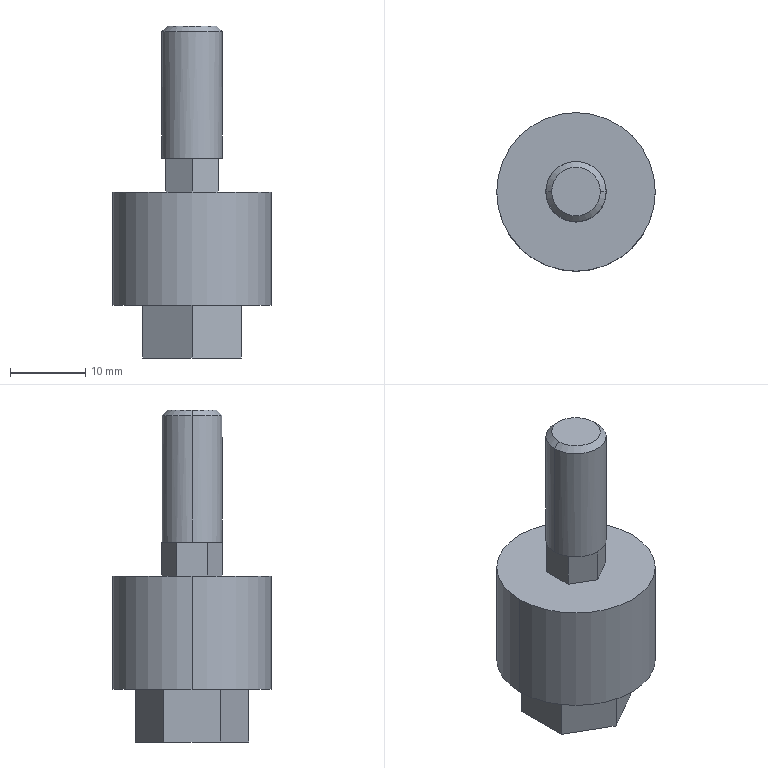Part | NX | features BREP 1 | 1 solid | 39 faces | box 21 x 21 x 44 mm | volume 7001 mm3 | plane 29 | cylinder 6 | cone 4 | commonest cylinder face diameters 6.647 x2 8 x2 21 x2
STEP:
#1=CARTESIAN_POINT('',(-10.5,0.,22.));
#2=VERTEX_POINT('',#1);
#3=CARTESIAN_POINT('',(10.5,0.,22.));
#4=VERTEX_POINT('',#3);
#5=CARTESIAN_POINT('',(0.,0.,22.));
#6=DIRECTION('',(0.,0.,-1.));
#7=DIRECTION('',(-1.,0.,0.));
#8=AXIS2_PLACEMENT_3D('',#5,#6,#7);
#9=CIRCLE('',#8,10.5);
#10=EDGE_CURVE('',#2,#4,#9,.T.);
#11=ORIENTED_EDGE('',*,*,#10,.T.);
#12=CARTESIAN_POINT('',(10.5,0.,7.));
#13=VERTEX_POINT('',#12);
#14=CARTESIAN_POINT('',(10.5,0.,14.5));
#15=DIRECTION('',(0.,0.,-1.));
#16=VECTOR('',#15,1000.);
#17=LINE('',#14,#16);
#18=EDGE_CURVE('',#4,#13,#17,.T.);
#19=ORIENTED_EDGE('',*,*,#18,.T.);
#20=CARTESIAN_POINT('',(-10.5,0.,7.));
#21=VERTEX_POINT('',#20);
#22=CARTESIAN_POINT('',(0.,0.,7.));
#23=DIRECTION('',(0.,0.,1.));
#24=DIRECTION('',(-1.,0.,0.));
#25=AXIS2_PLACEMENT_3D('',#22,#23,#24);
#26=CIRCLE('',#25,10.5);
#27=EDGE_CURVE('',#13,#21,#26,.T.);
#28=ORIENTED_EDGE('',*,*,#27,.T.);
#29=CARTESIAN_POINT('',(-10.5,0.,14.5));
#30=DIRECTION('',(0.,0.,-1.));
#31=VECTOR('',#30,1000.);
#32=LINE('',#29,#31);
#33=EDGE_CURVE('',#2,#21,#32,.T.);
#34=ORIENTED_EDGE('',*,*,#33,.F.);
#35=EDGE_LOOP('',(#11,#19,#28,#34));
#36=FACE_BOUND('',#35,.T.);
#37=CARTESIAN_POINT('',(0.,0.,14.5));
#38=DIRECTION('',(0.,0.,-1.));
#39=DIRECTION('',(-1.,0.,0.));
#40=AXIS2_PLACEMENT_3D('',#37,#38,#39);
#41=CYLINDRICAL_SURFACE('',#40,10.5);
#42=ADVANCED_FACE('',(#36),#41,.T.);
#43=CARTESIAN_POINT('',(-4.,0.,43.233));
#44=VERTEX_POINT('',#43);
#45=CARTESIAN_POINT('',(4.,0.,43.233));
#46=VERTEX_POINT('',#45);
#47=CARTESIAN_POINT('',(0.,0.,43.233));
#48=DIRECTION('',(0.,0.,-1.));
#49=DIRECTION('',(-1.,0.,0.));
#50=AXIS2_PLACEMENT_3D('',#47,#48,#49);
#51=CIRCLE('',#50,4.);
#52=EDGE_CURVE('',#44,#46,#51,.T.);
#53=ORIENTED_EDGE('',*,*,#52,.T.);
#54=CARTESIAN_POINT('',(4.,0.,26.5));
#55=VERTEX_POINT('',#54);
#56=CARTESIAN_POINT('',(4.,0.,34.867));
#57=DIRECTION('',(0.,0.,-1.));
#58=VECTOR('',#57,1000.);
#59=LINE('',#56,#58);
#60=EDGE_CURVE('',#46,#55,#59,.T.);
#61=ORIENTED_EDGE('',*,*,#60,.T.);
#62=CARTESIAN_POINT('',(3.5,1.936,26.5));
#63=VERTEX_POINT('',#62);
#64=CARTESIAN_POINT('',(0.,0.,26.5));
#65=DIRECTION('',(0.,0.,-1.));
#66=DIRECTION('',(-1.,0.,0.));
#67=AXIS2_PLACEMENT_3D('',#64,#65,#66);
#68=CIRCLE('',#67,4.);
#69=EDGE_CURVE('',#63,#55,#68,.T.);
#70=ORIENTED_EDGE('',*,*,#69,.F.);
#71=CARTESIAN_POINT('',(3.427,2.063,26.5));
#72=VERTEX_POINT('',#71);
#73=CARTESIAN_POINT('',(0.,0.,26.5));
#74=DIRECTION('',(0.,0.,-1.));
#75=DIRECTION('',(1.,0.,0.));
#76=AXIS2_PLACEMENT_3D('',#73,#74,#75);
#77=CIRCLE('',#76,4.);
#78=EDGE_CURVE('',#72,#63,#77,.T.);
#79=ORIENTED_EDGE('',*,*,#78,.F.);
#80=CARTESIAN_POINT('',(0.07295,3.999,26.5));
#81=VERTEX_POINT('',#80);
#82=CARTESIAN_POINT('',(0.,0.,26.5));
#83=DIRECTION('',(0.,0.,-1.));
#84=DIRECTION('',(-1.,0.,0.));
#85=AXIS2_PLACEMENT_3D('',#82,#83,#84);
#86=CIRCLE('',#85,4.);
#87=EDGE_CURVE('',#81,#72,#86,.T.);
#88=ORIENTED_EDGE('',*,*,#87,.F.);
#89=CARTESIAN_POINT('',(-0.07295,3.999,26.5));
#90=VERTEX_POINT('',#89);
#91=CARTESIAN_POINT('',(0.,0.,26.5));
#92=DIRECTION('',(0.,0.,-1.));
#93=DIRECTION('',(1.,0.,0.));
#94=AXIS2_PLACEMENT_3D('',#91,#92,#93);
#95=CIRCLE('',#94,4.);
#96=EDGE_CURVE('',#90,#81,#95,.T.);
#97=ORIENTED_EDGE('',*,*,#96,.F.);
#98=CARTESIAN_POINT('',(-3.427,2.063,26.5));
#99=VERTEX_POINT('',#98);
#100=CARTESIAN_POINT('',(0.,0.,26.5));
#101=DIRECTION('',(0.,0.,-1.));
#102=DIRECTION('',(-1.,0.,0.));
#103=AXIS2_PLACEMENT_3D('',#100,#101,#102);
#104=CIRCLE('',#103,4.);
#105=EDGE_CURVE('',#99,#90,#104,.T.);
#106=ORIENTED_EDGE('',*,*,#105,.F.);
#107=CARTESIAN_POINT('',(-3.5,1.936,26.5));
#108=VERTEX_POINT('',#107);
#109=CARTESIAN_POINT('',(0.,0.,26.5));
#110=DIRECTION('',(0.,0.,-1.));
#111=DIRECTION('',(1.,0.,0.));
#112=AXIS2_PLACEMENT_3D('',#109,#110,#111);
#113=CIRCLE('',#112,4.);
#114=EDGE_CURVE('',#108,#99,#113,.T.);
#115=ORIENTED_EDGE('',*,*,#114,.F.);
#116=CARTESIAN_POINT('',(-4.,0.,26.5));
#117=VERTEX_POINT('',#116);
#118=CARTESIAN_POINT('',(0.,0.,26.5));
#119=DIRECTION('',(0.,0.,-1.));
#120=DIRECTION('',(-1.,0.,0.));
#121=AXIS2_PLACEMENT_3D('',#118,#119,#120);
#122=CIRCLE('',#121,4.);
#123=EDGE_CURVE('',#117,#108,#122,.T.);
#124=ORIENTED_EDGE('',*,*,#123,.F.);
#125=CARTESIAN_POINT('',(-4.,0.,34.867));
#126=DIRECTION('',(0.,0.,-1.));
#127=VECTOR('',#126,1000.);
#128=LINE('',#125,#127);
#129=EDGE_CURVE('',#44,#117,#128,.T.);
#130=ORIENTED_EDGE('',*,*,#129,.F.);
#131=EDGE_LOOP('',(#53,#61,#70,#79,#88,#97,#106,#115,#124,#130));
#132=FACE_BOUND('',#131,.T.);
#133=CARTESIAN_POINT('',(0.,0.,34.867));
#134=DIRECTION('',(0.,0.,-1.));
#135=DIRECTION('',(-1.,0.,0.));
#136=AXIS2_PLACEMENT_3D('',#133,#134,#135);
#137=CYLINDRICAL_SURFACE('',#136,4.);
#138=ADVANCED_FACE('',(#132),#137,.T.);
#139=CARTESIAN_POINT('',(3.324,0.,0.6765));
#140=VERTEX_POINT('',#139);
#141=CARTESIAN_POINT('',(-3.324,0.,0.6765));
#142=VERTEX_POINT('',#141);
#143=CARTESIAN_POINT('',(0.,0.,0.6765));
#144=DIRECTION('',(0.,0.,-1.));
#145=DIRECTION('',(0.,1.,0.));
#146=AXIS2_PLACEMENT_3D('',#143,#144,#145);
#147=CIRCLE('',#146,3.324);
#148=EDGE_CURVE('',#140,#142,#147,.T.);
#149=ORIENTED_EDGE('',*,*,#148,.F.);
#150=CARTESIAN_POINT('',(4.,0.,0.));
#151=VERTEX_POINT('',#150);
#152=CARTESIAN_POINT('',(4.,0.,0.));
#153=DIRECTION('',(0.7071,0.,-0.7071));
#154=VECTOR('',#153,1000.);
#155=LINE('',#152,#154);
#156=EDGE_CURVE('',#140,#151,#155,.T.);
#157=ORIENTED_EDGE('',*,*,#156,.T.);
#158=CARTESIAN_POINT('',(-4.,0.,0.));
#159=VERTEX_POINT('',#158);
#160=CARTESIAN_POINT('',(0.,0.,0.));
#161=DIRECTION('',(0.,0.,1.));
#162=DIRECTION('',(-1.,0.,0.));
#163=AXIS2_PLACEMENT_3D('',#160,#161,#162);
#164=CIRCLE('',#163,4.);
#165=EDGE_CURVE('',#159,#151,#164,.T.);
#166=ORIENTED_EDGE('',*,*,#165,.F.);
#167=CARTESIAN_POINT('',(-4.,0.,0.));
#168=DIRECTION('',(-0.7071,0.,-0.7071));
#169=VECTOR('',#168,1000.);
#170=LINE('',#167,#169);
#171=EDGE_CURVE('',#142,#159,#170,.T.);
#172=ORIENTED_EDGE('',*,*,#171,.F.);
#173=EDGE_LOOP('',(#149,#157,#166,#172));
#174=FACE_BOUND('',#173,.T.);
#175=CARTESIAN_POINT('',(0.,0.,0.));
#176=DIRECTION('',(0.,0.,-1.));
#177=DIRECTION('',(-1.,0.,0.));
#178=AXIS2_PLACEMENT_3D('',#175,#176,#177);
#179=CONICAL_SURFACE('',#178,4.,0.7854);
#180=ADVANCED_FACE('',(#174),#179,.F.);
#181=CARTESIAN_POINT('',(-3.233,0.,44.));
#182=VERTEX_POINT('',#181);
#183=CARTESIAN_POINT('',(3.233,0.,44.));
#184=VERTEX_POINT('',#183);
#185=CARTESIAN_POINT('',(0.,0.,44.));
#186=DIRECTION('',(0.,0.,-1.));
#187=DIRECTION('',(-1.,0.,0.));
#188=AXIS2_PLACEMENT_3D('',#185,#186,#187);
#189=CIRCLE('',#188,3.233);
#190=EDGE_CURVE('',#182,#184,#189,.T.);
#191=ORIENTED_EDGE('',*,*,#190,.T.);
#192=CARTESIAN_POINT('',(4.,0.,43.233));
#193=DIRECTION('',(0.7071,0.,-0.7071));
#194=VECTOR('',#193,1000.);
#195=LINE('',#192,#194);
#196=EDGE_CURVE('',#184,#46,#195,.T.);
#197=ORIENTED_EDGE('',*,*,#196,.T.);
#198=ORIENTED_EDGE('',*,*,#52,.F.);
#199=CARTESIAN_POINT('',(-4.,0.,43.233));
#200=DIRECTION('',(-0.7071,0.,-0.7071));
#201=VECTOR('',#200,1000.);
#202=LINE('',#199,#201);
#203=EDGE_CURVE('',#182,#44,#202,.T.);
#204=ORIENTED_EDGE('',*,*,#203,.F.);
#205=EDGE_LOOP('',(#191,#197,#198,#204));
#206=FACE_BOUND('',#205,.T.);
#207=CARTESIAN_POINT('',(0.,0.,43.233));
#208=DIRECTION('',(0.,0.,-1.));
#209=DIRECTION('',(-1.,0.,0.));
#210=AXIS2_PLACEMENT_3D('',#207,#208,#209);
#211=CONICAL_SURFACE('',#210,4.,0.7854);
#212=ADVANCED_FACE('',(#206),#211,.T.);
#213=CARTESIAN_POINT('',(3.324,0.,8.));
#214=VERTEX_POINT('',#213);
#215=CARTESIAN_POINT('',(-3.324,0.,8.));
#216=VERTEX_POINT('',#215);
#217=CARTESIAN_POINT('',(0.,0.,8.));
#218=DIRECTION('',(0.,0.,-1.));
#219=DIRECTION('',(-1.,0.,0.));
#220=AXIS2_PLACEMENT_3D('',#217,#218,#219);
#221=CIRCLE('',#220,3.324);
#222=EDGE_CURVE('',#214,#216,#221,.T.);
#223=ORIENTED_EDGE('',*,*,#222,.F.);
#224=CARTESIAN_POINT('',(3.324,0.,4.338));
#225=DIRECTION('',(0.,0.,-1.));
#226=VECTOR('',#225,1000.);
#227=LINE('',#224,#226);
#228=EDGE_CURVE('',#214,#140,#227,.T.);
#229=ORIENTED_EDGE('',*,*,#228,.T.);
#230=ORIENTED_EDGE('',*,*,#148,.T.);
#231=CARTESIAN_POINT('',(-3.324,0.,4.338));
#232=DIRECTION('',(0.,0.,-1.));
#233=VECTOR('',#232,1000.);
#234=LINE('',#231,#233);
#235=EDGE_CURVE('',#216,#142,#234,.T.);
#236=ORIENTED_EDGE('',*,*,#235,.F.);
#237=EDGE_LOOP('',(#223,#229,#230,#236));
#238=FACE_BOUND('',#237,.T.);
#239=CARTESIAN_POINT('',(0.,0.,4.338));
#240=DIRECTION('',(0.,0.,-1.));
#241=DIRECTION('',(-1.,0.,0.));
#242=AXIS2_PLACEMENT_3D('',#239,#240,#241);
#243=CYLINDRICAL_SURFACE('',#242,3.324);
#244=ADVANCED_FACE('',(#238),#243,.F.);
#245=ORIENTED_EDGE('',*,*,#18,.F.);
#246=CARTESIAN_POINT('',(0.,0.,22.));
#247=DIRECTION('',(0.,0.,-1.));
#248=DIRECTION('',(-1.,0.,0.));
#249=AXIS2_PLACEMENT_3D('',#246,#247,#248);
#250=CIRCLE('',#249,10.5);
#251=EDGE_CURVE('',#4,#2,#250,.T.);
#252=ORIENTED_EDGE('',*,*,#251,.T.);
#253=ORIENTED_EDGE('',*,*,#33,.T.);
#254=CARTESIAN_POINT('',(0.,0.,7.));
#255=DIRECTION('',(0.,0.,1.));
#256=DIRECTION('',(-1.,0.,0.));
#257=AXIS2_PLACEMENT_3D('',#254,#255,#256);
#258=CIRCLE('',#257,10.5);
#259=EDGE_CURVE('',#21,#13,#258,.T.);
#260=ORIENTED_EDGE('',*,*,#259,.T.);
#261=EDGE_LOOP('',(#245,#252,#253,#260));
#262=FACE_BOUND('',#261,.T.);
#263=CARTESIAN_POINT('',(0.,0.,14.5));
#264=DIRECTION('',(0.,0.,-1.));
#265=DIRECTION('',(-1.,0.,0.));
#266=AXIS2_PLACEMENT_3D('',#263,#264,#265);
#267=CYLINDRICAL_SURFACE('',#266,10.5);
#268=ADVANCED_FACE('',(#262),#267,.T.);
#269=ORIENTED_EDGE('',*,*,#10,.F.);
#270=ORIENTED_EDGE('',*,*,#251,.F.);
#271=EDGE_LOOP('',(#269,#270));
#272=FACE_BOUND('',#271,.T.);
#273=CARTESIAN_POINT('',(3.5,2.021,22.));
#274=VERTEX_POINT('',#273);
#275=CARTESIAN_POINT('',(3.5,-2.021,22.));
#276=VERTEX_POINT('',#275);
#277=CARTESIAN_POINT('',(3.5,5.25,22.));
#278=DIRECTION('',(0.,-1.,0.));
#279=VECTOR('',#278,1000.);
#280=LINE('',#277,#279);
#281=EDGE_CURVE('',#274,#276,#280,.T.);
#282=ORIENTED_EDGE('',*,*,#281,.T.);
#283=CARTESIAN_POINT('',(0.,-4.041,22.));
#284=VERTEX_POINT('',#283);
#285=CARTESIAN_POINT('',(3.5,-2.021,22.));
#286=DIRECTION('',(-0.866,-0.5,0.));
#287=VECTOR('',#286,1000.);
#288=LINE('',#285,#287);
#289=EDGE_CURVE('',#276,#284,#288,.T.);
#290=ORIENTED_EDGE('',*,*,#289,.T.);
#291=CARTESIAN_POINT('',(-3.5,-2.021,22.));
#292=VERTEX_POINT('',#291);
#293=CARTESIAN_POINT('',(0.,-4.041,22.));
#294=DIRECTION('',(-0.866,0.5,0.));
#295=VECTOR('',#294,1000.);
#296=LINE('',#293,#295);
#297=EDGE_CURVE('',#284,#292,#296,.T.);
#298=ORIENTED_EDGE('',*,*,#297,.T.);
#299=CARTESIAN_POINT('',(-3.5,2.021,22.));
#300=VERTEX_POINT('',#299);
#301=CARTESIAN_POINT('',(-3.5,5.25,22.));
#302=DIRECTION('',(0.,1.,0.));
#303=VECTOR('',#302,1000.);
#304=LINE('',#301,#303);
#305=EDGE_CURVE('',#292,#300,#304,.T.);
#306=ORIENTED_EDGE('',*,*,#305,.T.);
#307=CARTESIAN_POINT('',(0.,4.041,22.));
#308=VERTEX_POINT('',#307);
#309=CARTESIAN_POINT('',(-3.5,2.021,22.));
#310=DIRECTION('',(0.866,0.5,0.));
#311=VECTOR('',#310,1000.);
#312=LINE('',#309,#311);
#313=EDGE_CURVE('',#300,#308,#312,.T.);
#314=ORIENTED_EDGE('',*,*,#313,.T.);
#315=CARTESIAN_POINT('',(0.,4.041,22.));
#316=DIRECTION('',(0.866,-0.5,0.));
#317=VECTOR('',#316,1000.);
#318=LINE('',#315,#317);
#319=EDGE_CURVE('',#308,#274,#318,.T.);
#320=ORIENTED_EDGE('',*,*,#319,.T.);
#321=EDGE_LOOP('',(#282,#290,#298,#306,#314,#320));
#322=FACE_BOUND('',#321,.T.);
#323=CARTESIAN_POINT('',(0.,5.25,22.));
#324=DIRECTION('',(0.,0.,1.));
#325=DIRECTION('',(1.,0.,0.));
#326=AXIS2_PLACEMENT_3D('',#323,#324,#325);
#327=PLANE('',#326);
#328=ADVANCED_FACE('',(#272,#322),#327,.T.);
#329=ORIENTED_EDGE('',*,*,#259,.F.);
#330=ORIENTED_EDGE('',*,*,#27,.F.);
#331=EDGE_LOOP('',(#329,#330));
#332=FACE_BOUND('',#331,.T.);
#333=CARTESIAN_POINT('',(6.5,3.753,7.));
#334=VERTEX_POINT('',#333);
#335=CARTESIAN_POINT('',(0.,7.506,7.));
#336=VERTEX_POINT('',#335);
#337=CARTESIAN_POINT('',(6.5,3.753,7.));
#338=DIRECTION('',(-0.866,0.5,0.));
#339=VECTOR('',#338,1000.);
#340=LINE('',#337,#339);
#341=EDGE_CURVE('',#334,#336,#340,.T.);
#342=ORIENTED_EDGE('',*,*,#341,.T.);
#343=CARTESIAN_POINT('',(-6.5,3.753,7.));
#344=VERTEX_POINT('',#343);
#345=CARTESIAN_POINT('',(0.,7.506,7.));
#346=DIRECTION('',(-0.866,-0.5,0.));
#347=VECTOR('',#346,1000.);
#348=LINE('',#345,#347);
#349=EDGE_CURVE('',#336,#344,#348,.T.);
#350=ORIENTED_EDGE('',*,*,#349,.T.);
#351=CARTESIAN_POINT('',(-6.5,-3.753,7.));
#352=VERTEX_POINT('',#351);
#353=CARTESIAN_POINT('',(-6.5,9.15,7.));
#354=DIRECTION('',(0.,-1.,0.));
#355=VECTOR('',#354,1000.);
#356=LINE('',#353,#355);
#357=EDGE_CURVE('',#344,#352,#356,.T.);
#358=ORIENTED_EDGE('',*,*,#357,.T.);
#359=CARTESIAN_POINT('',(0.,-7.506,7.));
#360=VERTEX_POINT('',#359);
#361=CARTESIAN_POINT('',(-6.5,-3.753,7.));
#362=DIRECTION('',(0.866,-0.5,0.));
#363=VECTOR('',#362,1000.);
#364=LINE('',#361,#363);
#365=EDGE_CURVE('',#352,#360,#364,.T.);
#366=ORIENTED_EDGE('',*,*,#365,.T.);
#367=CARTESIAN_POINT('',(6.5,-3.753,7.));
#368=VERTEX_POINT('',#367);
#369=CARTESIAN_POINT('',(0.,-7.506,7.));
#370=DIRECTION('',(0.866,0.5,0.));
#371=VECTOR('',#370,1000.);
#372=LINE('',#369,#371);
#373=EDGE_CURVE('',#360,#368,#372,.T.);
#374=ORIENTED_EDGE('',*,*,#373,.T.);
#375=CARTESIAN_POINT('',(6.5,9.15,7.));
#376=DIRECTION('',(0.,1.,0.));
#377=VECTOR('',#376,1000.);
#378=LINE('',#375,#377);
#379=EDGE_CURVE('',#368,#334,#378,.T.);
#380=ORIENTED_EDGE('',*,*,#379,.T.);
#381=EDGE_LOOP('',(#342,#350,#358,#366,#374,#380));
#382=FACE_BOUND('',#381,.T.);
#383=CARTESIAN_POINT('',(0.,9.15,7.));
#384=DIRECTION('',(0.,0.,-1.));
#385=DIRECTION('',(0.,-1.,0.));
#386=AXIS2_PLACEMENT_3D('',#383,#384,#385);
#387=PLANE('',#386);
#388=ADVANCED_FACE('',(#332,#382),#387,.T.);
#389=CARTESIAN_POINT('',(0.07295,-3.999,26.5));
#390=VERTEX_POINT('',#389);
#391=CARTESIAN_POINT('',(0.,-4.041,26.5));
#392=VERTEX_POINT('',#391);
#393=CARTESIAN_POINT('',(0.,-4.041,26.5));
#394=DIRECTION('',(-0.866,-0.5,0.));
#395=VECTOR('',#394,1000.);
#396=LINE('',#393,#395);
#397=EDGE_CURVE('',#390,#392,#396,.T.);
#398=ORIENTED_EDGE('',*,*,#397,.T.);
#399=CARTESIAN_POINT('',(0.,-4.041,26.5));
#400=DIRECTION('',(0.,0.,-1.));
#401=VECTOR('',#400,1000.);
#402=LINE('',#399,#401);
#403=EDGE_CURVE('',#392,#284,#402,.T.);
#404=ORIENTED_EDGE('',*,*,#403,.T.);
#405=ORIENTED_EDGE('',*,*,#289,.F.);
#406=CARTESIAN_POINT('',(3.5,-2.021,26.5));
#407=VERTEX_POINT('',#406);
#408=CARTESIAN_POINT('',(3.5,-2.021,26.5));
#409=DIRECTION('',(0.,0.,1.));
#410=VECTOR('',#409,1000.);
#411=LINE('',#408,#410);
#412=EDGE_CURVE('',#276,#407,#411,.T.);
#413=ORIENTED_EDGE('',*,*,#412,.T.);
#414=CARTESIAN_POINT('',(3.427,-2.063,26.5));
#415=VERTEX_POINT('',#414);
#416=CARTESIAN_POINT('',(0.,-4.041,26.5));
#417=DIRECTION('',(-0.866,-0.5,0.));
#418=VECTOR('',#417,1000.);
#419=LINE('',#416,#418);
#420=EDGE_CURVE('',#407,#415,#419,.T.);
#421=ORIENTED_EDGE('',*,*,#420,.T.);
#422=CARTESIAN_POINT('',(0.,-4.041,26.5));
#423=DIRECTION('',(-0.866,-0.5,0.));
#424=VECTOR('',#423,1000.);
#425=LINE('',#422,#424);
#426=EDGE_CURVE('',#415,#390,#425,.T.);
#427=ORIENTED_EDGE('',*,*,#426,.T.);
#428=EDGE_LOOP('',(#398,#404,#405,#413,#421,#427));
#429=FACE_BOUND('',#428,.T.);
#430=CARTESIAN_POINT('',(0.,-4.041,26.5));
#431=DIRECTION('',(0.5,-0.866,0.));
#432=DIRECTION('',(0.,0.,-1.));
#433=AXIS2_PLACEMENT_3D('',#430,#431,#432);
#434=PLANE('',#433);
#435=ADVANCED_FACE('',(#429),#434,.T.);
#436=CARTESIAN_POINT('',(3.5,-1.936,26.5));
#437=VERTEX_POINT('',#436);
#438=CARTESIAN_POINT('',(3.5,-2.021,26.5));
#439=DIRECTION('',(0.,-1.,0.));
#440=VECTOR('',#439,1000.);
#441=LINE('',#438,#440);
#442=EDGE_CURVE('',#437,#407,#441,.T.);
#443=ORIENTED_EDGE('',*,*,#442,.T.);
#444=ORIENTED_EDGE('',*,*,#412,.F.);
#445=ORIENTED_EDGE('',*,*,#281,.F.);
#446=CARTESIAN_POINT('',(3.5,2.021,26.5));
#447=VERTEX_POINT('',#446);
#448=CARTESIAN_POINT('',(3.5,2.021,26.5));
#449=DIRECTION('',(0.,0.,1.));
#450=VECTOR('',#449,1000.);
#451=LINE('',#448,#450);
#452=EDGE_CURVE('',#274,#447,#451,.T.);
#453=ORIENTED_EDGE('',*,*,#452,.T.);
#454=CARTESIAN_POINT('',(3.5,-2.021,26.5));
#455=DIRECTION('',(0.,-1.,0.));
#456=VECTOR('',#455,1000.);
#457=LINE('',#454,#456);
#458=EDGE_CURVE('',#447,#63,#457,.T.);
#459=ORIENTED_EDGE('',*,*,#458,.T.);
#460=CARTESIAN_POINT('',(3.5,-2.021,26.5));
#461=DIRECTION('',(0.,-1.,0.));
#462=VECTOR('',#461,1000.);
#463=LINE('',#460,#462);
#464=EDGE_CURVE('',#63,#437,#463,.T.);
#465=ORIENTED_EDGE('',*,*,#464,.T.);
#466=EDGE_LOOP('',(#443,#444,#445,#453,#459,#465));
#467=FACE_BOUND('',#466,.T.);
#468=CARTESIAN_POINT('',(3.5,-2.021,26.5));
#469=DIRECTION('',(1.,0.,0.));
#470=DIRECTION('',(0.,1.,0.));
#471=AXIS2_PLACEMENT_3D('',#468,#469,#470);
#472=PLANE('',#471);
#473=ADVANCED_FACE('',(#467),#472,.T.);
#474=CARTESIAN_POINT('',(3.5,2.021,26.5));
#475=DIRECTION('',(0.866,-0.5,0.));
#476=VECTOR('',#475,1000.);
#477=LINE('',#474,#476);
#478=EDGE_CURVE('',#72,#447,#477,.T.);
#479=ORIENTED_EDGE('',*,*,#478,.T.);
#480=ORIENTED_EDGE('',*,*,#452,.F.);
#481=ORIENTED_EDGE('',*,*,#319,.F.);
#482=CARTESIAN_POINT('',(0.,4.041,26.5));
#483=VERTEX_POINT('',#482);
#484=CARTESIAN_POINT('',(0.,4.041,26.5));
#485=DIRECTION('',(0.,0.,1.));
#486=VECTOR('',#485,1000.);
#487=LINE('',#484,#486);
#488=EDGE_CURVE('',#308,#483,#487,.T.);
#489=ORIENTED_EDGE('',*,*,#488,.T.);
#490=CARTESIAN_POINT('',(3.5,2.021,26.5));
#491=DIRECTION('',(0.866,-0.5,0.));
#492=VECTOR('',#491,1000.);
#493=LINE('',#490,#492);
#494=EDGE_CURVE('',#483,#81,#493,.T.);
#495=ORIENTED_EDGE('',*,*,#494,.T.);
#496=CARTESIAN_POINT('',(3.5,2.021,26.5));
#497=DIRECTION('',(0.866,-0.5,0.));
#498=VECTOR('',#497,1000.);
#499=LINE('',#496,#498);
#500=EDGE_CURVE('',#81,#72,#499,.T.);
#501=ORIENTED_EDGE('',*,*,#500,.T.);
#502=EDGE_LOOP('',(#479,#480,#481,#489,#495,#501));
#503=FACE_BOUND('',#502,.T.);
#504=CARTESIAN_POINT('',(3.5,2.021,26.5));
#505=DIRECTION('',(0.5,0.866,0.));
#506=DIRECTION('',(0.,0.,-1.));
#507=AXIS2_PLACEMENT_3D('',#504,#505,#506);
#508=PLANE('',#507);
#509=ADVANCED_FACE('',(#503),#508,.T.);
#510=CARTESIAN_POINT('',(0.,4.041,26.5));
#511=DIRECTION('',(0.866,0.5,0.));
#512=VECTOR('',#511,1000.);
#513=LINE('',#510,#512);
#514=EDGE_CURVE('',#90,#483,#513,.T.);
#515=ORIENTED_EDGE('',*,*,#514,.T.);
#516=ORIENTED_EDGE('',*,*,#488,.F.);
#517=ORIENTED_EDGE('',*,*,#313,.F.);
#518=CARTESIAN_POINT('',(-3.5,2.021,26.5));
#519=VERTEX_POINT('',#518);
#520=CARTESIAN_POINT('',(-3.5,2.021,26.5));
#521=DIRECTION('',(0.,0.,1.));
#522=VECTOR('',#521,1000.);
#523=LINE('',#520,#522);
#524=EDGE_CURVE('',#300,#519,#523,.T.);
#525=ORIENTED_EDGE('',*,*,#524,.T.);
#526=CARTESIAN_POINT('',(0.,4.041,26.5));
#527=DIRECTION('',(0.866,0.5,0.));
#528=VECTOR('',#527,1000.);
#529=LINE('',#526,#528);
#530=EDGE_CURVE('',#519,#99,#529,.T.);
#531=ORIENTED_EDGE('',*,*,#530,.T.);
#532=CARTESIAN_POINT('',(0.,4.041,26.5));
#533=DIRECTION('',(0.866,0.5,0.));
#534=VECTOR('',#533,1000.);
#535=LINE('',#532,#534);
#536=EDGE_CURVE('',#99,#90,#535,.T.);
#537=ORIENTED_EDGE('',*,*,#536,.T.);
#538=EDGE_LOOP('',(#515,#516,#517,#525,#531,#537));
#539=FACE_BOUND('',#538,.T.);
#540=CARTESIAN_POINT('',(0.,4.041,26.5));
#541=DIRECTION('',(-0.5,0.866,0.));
#542=DIRECTION('',(0.,0.,1.));
#543=AXIS2_PLACEMENT_3D('',#540,#541,#542);
#544=PLANE('',#543);
#545=ADVANCED_FACE('',(#539),#544,.T.);
#546=CARTESIAN_POINT('',(-3.5,2.021,26.5));
#547=DIRECTION('',(0.,1.,0.));
#548=VECTOR('',#547,1000.);
#549=LINE('',#546,#548);
#550=EDGE_CURVE('',#108,#519,#549,.T.);
#551=ORIENTED_EDGE('',*,*,#550,.T.);
#552=ORIENTED_EDGE('',*,*,#524,.F.);
#553=ORIENTED_EDGE('',*,*,#305,.F.);
#554=CARTESIAN_POINT('',(-3.5,-2.021,26.5));
#555=VERTEX_POINT('',#554);
#556=CARTESIAN_POINT('',(-3.5,-2.021,26.5));
#557=DIRECTION('',(0.,0.,1.));
#558=VECTOR('',#557,1000.);
#559=LINE('',#556,#558);
#560=EDGE_CURVE('',#292,#555,#559,.T.);
#561=ORIENTED_EDGE('',*,*,#560,.T.);
#562=CARTESIAN_POINT('',(-3.5,-1.936,26.5));
#563=VERTEX_POINT('',#562);
#564=CARTESIAN_POINT('',(-3.5,2.021,26.5));
#565=DIRECTION('',(0.,1.,0.));
#566=VECTOR('',#565,1000.);
#567=LINE('',#564,#566);
#568=EDGE_CURVE('',#555,#563,#567,.T.);
#569=ORIENTED_EDGE('',*,*,#568,.T.);
#570=CARTESIAN_POINT('',(-3.5,2.021,26.5));
#571=DIRECTION('',(0.,1.,0.));
#572=VECTOR('',#571,1000.);
#573=LINE('',#570,#572);
#574=EDGE_CURVE('',#563,#108,#573,.T.);
#575=ORIENTED_EDGE('',*,*,#574,.T.);
#576=EDGE_LOOP('',(#551,#552,#553,#561,#569,#575));
#577=FACE_BOUND('',#576,.T.);
#578=CARTESIAN_POINT('',(-3.5,2.021,26.5));
#579=DIRECTION('',(-1.,0.,0.));
#580=DIRECTION('',(0.,0.,1.));
#581=AXIS2_PLACEMENT_3D('',#578,#579,#580);
#582=PLANE('',#581);
#583=ADVANCED_FACE('',(#577),#582,.T.);
#584=CARTESIAN_POINT('',(-3.427,-2.063,26.5));
#585=VERTEX_POINT('',#584);
#586=CARTESIAN_POINT('',(-3.5,-2.021,26.5));
#587=DIRECTION('',(-0.866,0.5,0.));
#588=VECTOR('',#587,1000.);
#589=LINE('',#586,#588);
#590=EDGE_CURVE('',#585,#555,#589,.T.);
#591=ORIENTED_EDGE('',*,*,#590,.T.);
#592=ORIENTED_EDGE('',*,*,#560,.F.);
#593=ORIENTED_EDGE('',*,*,#297,.F.);
#594=ORIENTED_EDGE('',*,*,#403,.F.);
#595=CARTESIAN_POINT('',(-0.07295,-3.999,26.5));
#596=VERTEX_POINT('',#595);
#597=CARTESIAN_POINT('',(-3.5,-2.021,26.5));
#598=DIRECTION('',(-0.866,0.5,0.));
#599=VECTOR('',#598,1000.);
#600=LINE('',#597,#599);
#601=EDGE_CURVE('',#392,#596,#600,.T.);
#602=ORIENTED_EDGE('',*,*,#601,.T.);
#603=CARTESIAN_POINT('',(-3.5,-2.021,26.5));
#604=DIRECTION('',(-0.866,0.5,0.));
#605=VECTOR('',#604,1000.);
#606=LINE('',#603,#605);
#607=EDGE_CURVE('',#596,#585,#606,.T.);
#608=ORIENTED_EDGE('',*,*,#607,.T.);
#609=EDGE_LOOP('',(#591,#592,#593,#594,#602,#608));
#610=FACE_BOUND('',#609,.T.);
#611=CARTESIAN_POINT('',(-3.5,-2.021,26.5));
#612=DIRECTION('',(-0.5,-0.866,0.));
#613=DIRECTION('',(-0.866,0.5,0.));
#614=AXIS2_PLACEMENT_3D('',#611,#612,#613);
#615=PLANE('',#614);
#616=ADVANCED_FACE('',(#610),#615,.T.);
#617=CARTESIAN_POINT('',(0.,7.506,0.));
#618=VERTEX_POINT('',#617);
#619=CARTESIAN_POINT('',(0.,7.506,0.));
#620=DIRECTION('',(0.,0.,1.));
#621=VECTOR('',#620,1000.);
#622=LINE('',#619,#621);
#623=EDGE_CURVE('',#618,#336,#622,.T.);
#624=ORIENTED_EDGE('',*,*,#623,.F.);
#625=CARTESIAN_POINT('',(-6.5,3.753,0.));
#626=VERTEX_POINT('',#625);
#627=CARTESIAN_POINT('',(0.,7.506,0.));
#628=DIRECTION('',(0.866,0.5,0.));
#629=VECTOR('',#628,1000.);
#630=LINE('',#627,#629);
#631=EDGE_CURVE('',#626,#618,#630,.T.);
#632=ORIENTED_EDGE('',*,*,#631,.F.);
#633=CARTESIAN_POINT('',(-6.5,3.753,0.));
#634=DIRECTION('',(0.,0.,-1.));
#635=VECTOR('',#634,1000.);
#636=LINE('',#633,#635);
#637=EDGE_CURVE('',#344,#626,#636,.T.);
#638=ORIENTED_EDGE('',*,*,#637,.F.);
#639=ORIENTED_EDGE('',*,*,#349,.F.);
#640=EDGE_LOOP('',(#624,#632,#638,#639));
#641=FACE_BOUND('',#640,.T.);
#642=CARTESIAN_POINT('',(0.,7.506,0.));
#643=DIRECTION('',(0.5,-0.866,0.));
#644=DIRECTION('',(0.,0.,-1.));
#645=AXIS2_PLACEMENT_3D('',#642,#643,#644);
#646=PLANE('',#645);
#647=ADVANCED_FACE('',(#641),#646,.F.);
#648=CARTESIAN_POINT('',(6.5,3.753,0.));
#649=VERTEX_POINT('',#648);
#650=CARTESIAN_POINT('',(6.5,3.753,0.));
#651=DIRECTION('',(0.,0.,1.));
#652=VECTOR('',#651,1000.);
#653=LINE('',#650,#652);
#654=EDGE_CURVE('',#649,#334,#653,.T.);
#655=ORIENTED_EDGE('',*,*,#654,.F.);
#656=CARTESIAN_POINT('',(6.5,3.753,0.));
#657=DIRECTION('',(0.866,-0.5,0.));
#658=VECTOR('',#657,1000.);
#659=LINE('',#656,#658);
#660=EDGE_CURVE('',#618,#649,#659,.T.);
#661=ORIENTED_EDGE('',*,*,#660,.F.);
#662=ORIENTED_EDGE('',*,*,#623,.T.);
#663=ORIENTED_EDGE('',*,*,#341,.F.);
#664=EDGE_LOOP('',(#655,#661,#662,#663));
#665=FACE_BOUND('',#664,.T.);
#666=CARTESIAN_POINT('',(6.5,3.753,0.));
#667=DIRECTION('',(-0.5,-0.866,0.));
#668=DIRECTION('',(-0.866,0.5,0.));
#669=AXIS2_PLACEMENT_3D('',#666,#667,#668);
#670=PLANE('',#669);
#671=ADVANCED_FACE('',(#665),#670,.F.);
#672=CARTESIAN_POINT('',(6.5,-3.753,0.));
#673=VERTEX_POINT('',#672);
#674=CARTESIAN_POINT('',(6.5,-3.753,0.));
#675=DIRECTION('',(0.,0.,1.));
#676=VECTOR('',#675,1000.);
#677=LINE('',#674,#676);
#678=EDGE_CURVE('',#673,#368,#677,.T.);
#679=ORIENTED_EDGE('',*,*,#678,.F.);
#680=CARTESIAN_POINT('',(6.5,-3.753,0.));
#681=DIRECTION('',(0.,-1.,0.));
#682=VECTOR('',#681,1000.);
#683=LINE('',#680,#682);
#684=EDGE_CURVE('',#649,#673,#683,.T.);
#685=ORIENTED_EDGE('',*,*,#684,.F.);
#686=ORIENTED_EDGE('',*,*,#654,.T.);
#687=ORIENTED_EDGE('',*,*,#379,.F.);
#688=EDGE_LOOP('',(#679,#685,#686,#687));
#689=FACE_BOUND('',#688,.T.);
#690=CARTESIAN_POINT('',(6.5,-3.753,0.));
#691=DIRECTION('',(-1.,0.,0.));
#692=DIRECTION('',(0.,0.,1.));
#693=AXIS2_PLACEMENT_3D('',#690,#691,#692);
#694=PLANE('',#693);
#695=ADVANCED_FACE('',(#689),#694,.F.);
#696=CARTESIAN_POINT('',(0.,-7.506,0.));
#697=VERTEX_POINT('',#696);
#698=CARTESIAN_POINT('',(0.,-7.506,0.));
#699=DIRECTION('',(0.,0.,1.));
#700=VECTOR('',#699,1000.);
#701=LINE('',#698,#700);
#702=EDGE_CURVE('',#697,#360,#701,.T.);
#703=ORIENTED_EDGE('',*,*,#702,.F.);
#704=CARTESIAN_POINT('',(0.,-7.506,0.));
#705=DIRECTION('',(-0.866,-0.5,0.));
#706=VECTOR('',#705,1000.);
#707=LINE('',#704,#706);
#708=EDGE_CURVE('',#673,#697,#707,.T.);
#709=ORIENTED_EDGE('',*,*,#708,.F.);
#710=ORIENTED_EDGE('',*,*,#678,.T.);
#711=ORIENTED_EDGE('',*,*,#373,.F.);
#712=EDGE_LOOP('',(#703,#709,#710,#711));
#713=FACE_BOUND('',#712,.T.);
#714=CARTESIAN_POINT('',(0.,-7.506,0.));
#715=DIRECTION('',(-0.5,0.866,0.));
#716=DIRECTION('',(0.,0.,1.));
#717=AXIS2_PLACEMENT_3D('',#714,#715,#716);
#718=PLANE('',#717);
#719=ADVANCED_FACE('',(#713),#718,.F.);
#720=CARTESIAN_POINT('',(-6.5,-3.753,0.));
#721=VERTEX_POINT('',#720);
#722=CARTESIAN_POINT('',(-6.5,-3.753,0.));
#723=DIRECTION('',(0.,0.,1.));
#724=VECTOR('',#723,1000.);
#725=LINE('',#722,#724);
#726=EDGE_CURVE('',#721,#352,#725,.T.);
#727=ORIENTED_EDGE('',*,*,#726,.F.);
#728=CARTESIAN_POINT('',(-6.5,-3.753,0.));
#729=DIRECTION('',(-0.866,0.5,0.));
#730=VECTOR('',#729,1000.);
#731=LINE('',#728,#730);
#732=EDGE_CURVE('',#697,#721,#731,.T.);
#733=ORIENTED_EDGE('',*,*,#732,.F.);
#734=ORIENTED_EDGE('',*,*,#702,.T.);
#735=ORIENTED_EDGE('',*,*,#365,.F.);
#736=EDGE_LOOP('',(#727,#733,#734,#735));
#737=FACE_BOUND('',#736,.T.);
#738=CARTESIAN_POINT('',(-6.5,-3.753,0.));
#739=DIRECTION('',(0.5,0.866,0.));
#740=DIRECTION('',(0.,0.,-1.));
#741=AXIS2_PLACEMENT_3D('',#738,#739,#740);
#742=PLANE('',#741);
#743=ADVANCED_FACE('',(#737),#742,.F.);
#744=ORIENTED_EDGE('',*,*,#637,.T.);
#745=CARTESIAN_POINT('',(-6.5,3.753,0.));
#746=DIRECTION('',(0.,1.,0.));
#747=VECTOR('',#746,1000.);
#748=LINE('',#745,#747);
#749=EDGE_CURVE('',#721,#626,#748,.T.);
#750=ORIENTED_EDGE('',*,*,#749,.F.);
#751=ORIENTED_EDGE('',*,*,#726,.T.);
#752=ORIENTED_EDGE('',*,*,#357,.F.);
#753=EDGE_LOOP('',(#744,#750,#751,#752));
#754=FACE_BOUND('',#753,.T.);
#755=CARTESIAN_POINT('',(-6.5,3.753,0.));
#756=DIRECTION('',(1.,0.,0.));
#757=DIRECTION('',(0.,1.,0.));
#758=AXIS2_PLACEMENT_3D('',#755,#756,#757);
#759=PLANE('',#758);
#760=ADVANCED_FACE('',(#754),#759,.F.);
#761=ORIENTED_EDGE('',*,*,#601,.F.);
#762=ORIENTED_EDGE('',*,*,#397,.F.);
#763=CARTESIAN_POINT('',(0.,0.,26.5));
#764=DIRECTION('',(0.,0.,1.));
#765=DIRECTION('',(-1.,0.,0.));
#766=AXIS2_PLACEMENT_3D('',#763,#764,#765);
#767=CIRCLE('',#766,4.);
#768=EDGE_CURVE('',#596,#390,#767,.T.);
#769=ORIENTED_EDGE('',*,*,#768,.F.);
#770=EDGE_LOOP('',(#761,#762,#769));
#771=FACE_BOUND('',#770,.T.);
#772=CARTESIAN_POINT('',(0.,0.,26.5));
#773=DIRECTION('',(0.,0.,1.));
#774=DIRECTION('',(1.,0.,0.));
#775=AXIS2_PLACEMENT_3D('',#772,#773,#774);
#776=PLANE('',#775);
#777=ADVANCED_FACE('',(#771),#776,.T.);
#778=ORIENTED_EDGE('',*,*,#426,.F.);
#779=CARTESIAN_POINT('',(0.,0.,26.5));
#780=DIRECTION('',(0.,0.,-1.));
#781=DIRECTION('',(-1.,0.,0.));
#782=AXIS2_PLACEMENT_3D('',#779,#780,#781);
#783=CIRCLE('',#782,4.);
#784=EDGE_CURVE('',#415,#390,#783,.T.);
#785=ORIENTED_EDGE('',*,*,#784,.T.);
#786=EDGE_LOOP('',(#778,#785));
#787=FACE_BOUND('',#786,.T.);
#788=CARTESIAN_POINT('',(0.,2.,26.5));
#789=DIRECTION('',(0.,0.,-1.));
#790=DIRECTION('',(0.,-1.,0.));
#791=AXIS2_PLACEMENT_3D('',#788,#789,#790);
#792=PLANE('',#791);
#793=ADVANCED_FACE('',(#787),#792,.T.);
#794=ORIENTED_EDGE('',*,*,#420,.F.);
#795=ORIENTED_EDGE('',*,*,#442,.F.);
#796=CARTESIAN_POINT('',(0.,0.,26.5));
#797=DIRECTION('',(0.,0.,-1.));
#798=DIRECTION('',(1.,0.,0.));
#799=AXIS2_PLACEMENT_3D('',#796,#797,#798);
#800=CIRCLE('',#799,4.);
#801=EDGE_CURVE('',#437,#415,#800,.T.);
#802=ORIENTED_EDGE('',*,*,#801,.T.);
#803=EDGE_LOOP('',(#794,#795,#802));
#804=FACE_BOUND('',#803,.T.);
#805=CARTESIAN_POINT('',(0.,0.,26.5));
#806=DIRECTION('',(0.,0.,1.));
#807=DIRECTION('',(1.,0.,0.));
#808=AXIS2_PLACEMENT_3D('',#805,#806,#807);
#809=PLANE('',#808);
#810=ADVANCED_FACE('',(#804),#809,.T.);
#811=ORIENTED_EDGE('',*,*,#464,.F.);
#812=ORIENTED_EDGE('',*,*,#69,.T.);
#813=CARTESIAN_POINT('',(0.,0.,26.5));
#814=DIRECTION('',(0.,0.,-1.));
#815=DIRECTION('',(-1.,0.,0.));
#816=AXIS2_PLACEMENT_3D('',#813,#814,#815);
#817=CIRCLE('',#816,4.);
#818=EDGE_CURVE('',#55,#437,#817,.T.);
#819=ORIENTED_EDGE('',*,*,#818,.T.);
#820=EDGE_LOOP('',(#811,#812,#819));
#821=FACE_BOUND('',#820,.T.);
#822=CARTESIAN_POINT('',(0.,2.,26.5));
#823=DIRECTION('',(0.,0.,-1.));
#824=DIRECTION('',(0.,-1.,0.));
#825=AXIS2_PLACEMENT_3D('',#822,#823,#824);
#826=PLANE('',#825);
#827=ADVANCED_FACE('',(#821),#826,.T.);
#828=ORIENTED_EDGE('',*,*,#458,.F.);
#829=ORIENTED_EDGE('',*,*,#478,.F.);
#830=ORIENTED_EDGE('',*,*,#78,.T.);
#831=EDGE_LOOP('',(#828,#829,#830));
#832=FACE_BOUND('',#831,.T.);
#833=CARTESIAN_POINT('',(0.,0.,26.5));
#834=DIRECTION('',(0.,0.,1.));
#835=DIRECTION('',(1.,0.,0.));
#836=AXIS2_PLACEMENT_3D('',#833,#834,#835);
#837=PLANE('',#836);
#838=ADVANCED_FACE('',(#832),#837,.T.);
#839=ORIENTED_EDGE('',*,*,#500,.F.);
#840=ORIENTED_EDGE('',*,*,#87,.T.);
#841=EDGE_LOOP('',(#839,#840));
#842=FACE_BOUND('',#841,.T.);
#843=CARTESIAN_POINT('',(0.,2.,26.5));
#844=DIRECTION('',(0.,0.,-1.));
#845=DIRECTION('',(0.,-1.,0.));
#846=AXIS2_PLACEMENT_3D('',#843,#844,#845);
#847=PLANE('',#846);
#848=ADVANCED_FACE('',(#842),#847,.T.);
#849=ORIENTED_EDGE('',*,*,#494,.F.);
#850=ORIENTED_EDGE('',*,*,#514,.F.);
#851=ORIENTED_EDGE('',*,*,#96,.T.);
#852=EDGE_LOOP('',(#849,#850,#851));
#853=FACE_BOUND('',#852,.T.);
#854=CARTESIAN_POINT('',(0.,0.,26.5));
#855=DIRECTION('',(0.,0.,1.));
#856=DIRECTION('',(1.,0.,0.));
#857=AXIS2_PLACEMENT_3D('',#854,#855,#856);
#858=PLANE('',#857);
#859=ADVANCED_FACE('',(#853),#858,.T.);
#860=ORIENTED_EDGE('',*,*,#536,.F.);
#861=ORIENTED_EDGE('',*,*,#105,.T.);
#862=EDGE_LOOP('',(#860,#861));
#863=FACE_BOUND('',#862,.T.);
#864=CARTESIAN_POINT('',(0.,2.,26.5));
#865=DIRECTION('',(0.,0.,-1.));
#866=DIRECTION('',(0.,-1.,0.));
#867=AXIS2_PLACEMENT_3D('',#864,#865,#866);
#868=PLANE('',#867);
#869=ADVANCED_FACE('',(#863),#868,.T.);
#870=ORIENTED_EDGE('',*,*,#530,.F.);
#871=ORIENTED_EDGE('',*,*,#550,.F.);
#872=ORIENTED_EDGE('',*,*,#114,.T.);
#873=EDGE_LOOP('',(#870,#871,#872));
#874=FACE_BOUND('',#873,.T.);
#875=CARTESIAN_POINT('',(0.,0.,26.5));
#876=DIRECTION('',(0.,0.,1.));
#877=DIRECTION('',(1.,0.,0.));
#878=AXIS2_PLACEMENT_3D('',#875,#876,#877);
#879=PLANE('',#878);
#880=ADVANCED_FACE('',(#874),#879,.T.);
#881=ORIENTED_EDGE('',*,*,#574,.F.);
#882=CARTESIAN_POINT('',(0.,0.,26.5));
#883=DIRECTION('',(0.,0.,-1.));
#884=DIRECTION('',(-1.,0.,0.));
#885=AXIS2_PLACEMENT_3D('',#882,#883,#884);
#886=CIRCLE('',#885,4.);
#887=EDGE_CURVE('',#563,#117,#886,.T.);
#888=ORIENTED_EDGE('',*,*,#887,.T.);
#889=ORIENTED_EDGE('',*,*,#123,.T.);
#890=EDGE_LOOP('',(#881,#888,#889));
#891=FACE_BOUND('',#890,.T.);
#892=CARTESIAN_POINT('',(0.,2.,26.5));
#893=DIRECTION('',(0.,0.,-1.));
#894=DIRECTION('',(0.,-1.,0.));
#895=AXIS2_PLACEMENT_3D('',#892,#893,#894);
#896=PLANE('',#895);
#897=ADVANCED_FACE('',(#891),#896,.T.);
#898=ORIENTED_EDGE('',*,*,#568,.F.);
#899=ORIENTED_EDGE('',*,*,#590,.F.);
#900=CARTESIAN_POINT('',(0.,0.,26.5));
#901=DIRECTION('',(0.,0.,-1.));
#902=DIRECTION('',(1.,0.,0.));
#903=AXIS2_PLACEMENT_3D('',#900,#901,#902);
#904=CIRCLE('',#903,4.);
#905=EDGE_CURVE('',#585,#563,#904,.T.);
#906=ORIENTED_EDGE('',*,*,#905,.T.);
#907=EDGE_LOOP('',(#898,#899,#906));
#908=FACE_BOUND('',#907,.T.);
#909=CARTESIAN_POINT('',(0.,0.,26.5));
#910=DIRECTION('',(0.,0.,1.));
#911=DIRECTION('',(1.,0.,0.));
#912=AXIS2_PLACEMENT_3D('',#909,#910,#911);
#913=PLANE('',#912);
#914=ADVANCED_FACE('',(#908),#913,.T.);
#915=ORIENTED_EDGE('',*,*,#607,.F.);
#916=CARTESIAN_POINT('',(0.,0.,26.5));
#917=DIRECTION('',(0.,0.,-1.));
#918=DIRECTION('',(-1.,0.,0.));
#919=AXIS2_PLACEMENT_3D('',#916,#917,#918);
#920=CIRCLE('',#919,4.);
#921=EDGE_CURVE('',#596,#585,#920,.T.);
#922=ORIENTED_EDGE('',*,*,#921,.T.);
#923=EDGE_LOOP('',(#915,#922));
#924=FACE_BOUND('',#923,.T.);
#925=CARTESIAN_POINT('',(0.,2.,26.5));
#926=DIRECTION('',(0.,0.,-1.));
#927=DIRECTION('',(0.,-1.,0.));
#928=AXIS2_PLACEMENT_3D('',#925,#926,#927);
#929=PLANE('',#928);
#930=ADVANCED_FACE('',(#924),#929,.T.);
#931=ORIENTED_EDGE('',*,*,#708,.T.);
#932=ORIENTED_EDGE('',*,*,#732,.T.);
#933=ORIENTED_EDGE('',*,*,#749,.T.);
#934=ORIENTED_EDGE('',*,*,#631,.T.);
#935=ORIENTED_EDGE('',*,*,#660,.T.);
#936=ORIENTED_EDGE('',*,*,#684,.T.);
#937=EDGE_LOOP('',(#931,#932,#933,#934,#935,#936));
#938=FACE_BOUND('',#937,.T.);
#939=ORIENTED_EDGE('',*,*,#165,.T.);
#940=CARTESIAN_POINT('',(0.,0.,0.));
#941=DIRECTION('',(0.,0.,1.));
#942=DIRECTION('',(-1.,0.,0.));
#943=AXIS2_PLACEMENT_3D('',#940,#941,#942);
#944=CIRCLE('',#943,4.);
#945=EDGE_CURVE('',#151,#159,#944,.T.);
#946=ORIENTED_EDGE('',*,*,#945,.T.);
#947=EDGE_LOOP('',(#939,#946));
#948=FACE_BOUND('',#947,.T.);
#949=CARTESIAN_POINT('',(0.,5.9,0.));
#950=DIRECTION('',(0.,0.,-1.));
#951=DIRECTION('',(0.,-1.,0.));
#952=AXIS2_PLACEMENT_3D('',#949,#950,#951);
#953=PLANE('',#952);
#954=ADVANCED_FACE('',(#938,#948),#953,.T.);
#955=ORIENTED_EDGE('',*,*,#60,.F.);
#956=CARTESIAN_POINT('',(0.,0.,43.233));
#957=DIRECTION('',(0.,0.,-1.));
#958=DIRECTION('',(-1.,0.,0.));
#959=AXIS2_PLACEMENT_3D('',#956,#957,#958);
#960=CIRCLE('',#959,4.);
#961=EDGE_CURVE('',#46,#44,#960,.T.);
#962=ORIENTED_EDGE('',*,*,#961,.T.);
#963=ORIENTED_EDGE('',*,*,#129,.T.);
#964=ORIENTED_EDGE('',*,*,#887,.F.);
#965=ORIENTED_EDGE('',*,*,#905,.F.);
#966=ORIENTED_EDGE('',*,*,#921,.F.);
#967=ORIENTED_EDGE('',*,*,#768,.T.);
#968=ORIENTED_EDGE('',*,*,#784,.F.);
#969=ORIENTED_EDGE('',*,*,#801,.F.);
#970=ORIENTED_EDGE('',*,*,#818,.F.);
#971=EDGE_LOOP('',(#955,#962,#963,#964,#965,#966,#967,#968,#969,#970));
#972=FACE_BOUND('',#971,.T.);
#973=CARTESIAN_POINT('',(0.,0.,34.867));
#974=DIRECTION('',(0.,0.,-1.));
#975=DIRECTION('',(-1.,0.,0.));
#976=AXIS2_PLACEMENT_3D('',#973,#974,#975);
#977=CYLINDRICAL_SURFACE('',#976,4.);
#978=ADVANCED_FACE('',(#972),#977,.T.);
#979=ORIENTED_EDGE('',*,*,#156,.F.);
#980=CARTESIAN_POINT('',(0.,0.,0.6765));
#981=DIRECTION('',(0.,0.,-1.));
#982=DIRECTION('',(0.,1.,0.));
#983=AXIS2_PLACEMENT_3D('',#980,#981,#982);
#984=CIRCLE('',#983,3.324);
#985=EDGE_CURVE('',#142,#140,#984,.T.);
#986=ORIENTED_EDGE('',*,*,#985,.F.);
#987=ORIENTED_EDGE('',*,*,#171,.T.);
#988=ORIENTED_EDGE('',*,*,#945,.F.);
#989=EDGE_LOOP('',(#979,#986,#987,#988));
#990=FACE_BOUND('',#989,.T.);
#991=CARTESIAN_POINT('',(0.,0.,0.));
#992=DIRECTION('',(0.,0.,-1.));
#993=DIRECTION('',(-1.,0.,0.));
#994=AXIS2_PLACEMENT_3D('',#991,#992,#993);
#995=CONICAL_SURFACE('',#994,4.,0.7854);
#996=ADVANCED_FACE('',(#990),#995,.F.);
#997=ORIENTED_EDGE('',*,*,#196,.F.);
#998=CARTESIAN_POINT('',(0.,0.,44.));
#999=DIRECTION('',(0.,0.,-1.));
#1000=DIRECTION('',(-1.,0.,0.));
#1001=AXIS2_PLACEMENT_3D('',#998,#999,#1000);
#1002=CIRCLE('',#1001,3.233);
#1003=EDGE_CURVE('',#184,#182,#1002,.T.);
#1004=ORIENTED_EDGE('',*,*,#1003,.T.);
#1005=ORIENTED_EDGE('',*,*,#203,.T.);
#1006=ORIENTED_EDGE('',*,*,#961,.F.);
#1007=EDGE_LOOP('',(#997,#1004,#1005,#1006));
#1008=FACE_BOUND('',#1007,.T.);
#1009=CARTESIAN_POINT('',(0.,0.,43.233));
#1010=DIRECTION('',(0.,0.,-1.));
#1011=DIRECTION('',(-1.,0.,0.));
#1012=AXIS2_PLACEMENT_3D('',#1009,#1010,#1011);
#1013=CONICAL_SURFACE('',#1012,4.,0.7854);
#1014=ADVANCED_FACE('',(#1008),#1013,.T.);
#1015=ORIENTED_EDGE('',*,*,#228,.F.);
#1016=CARTESIAN_POINT('',(0.,0.,8.));
#1017=DIRECTION('',(0.,0.,-1.));
#1018=DIRECTION('',(-1.,0.,0.));
#1019=AXIS2_PLACEMENT_3D('',#1016,#1017,#1018);
#1020=CIRCLE('',#1019,3.324);
#1021=EDGE_CURVE('',#216,#214,#1020,.T.);
#1022=ORIENTED_EDGE('',*,*,#1021,.F.);
#1023=ORIENTED_EDGE('',*,*,#235,.T.);
#1024=ORIENTED_EDGE('',*,*,#985,.T.);
#1025=EDGE_LOOP('',(#1015,#1022,#1023,#1024));
#1026=FACE_BOUND('',#1025,.T.);
#1027=CARTESIAN_POINT('',(0.,0.,4.338));
#1028=DIRECTION('',(0.,0.,-1.));
#1029=DIRECTION('',(-1.,0.,0.));
#1030=AXIS2_PLACEMENT_3D('',#1027,#1028,#1029);
#1031=CYLINDRICAL_SURFACE('',#1030,3.324);
#1032=ADVANCED_FACE('',(#1026),#1031,.F.);
#1033=ORIENTED_EDGE('',*,*,#190,.F.);
#1034=ORIENTED_EDGE('',*,*,#1003,.F.);
#1035=EDGE_LOOP('',(#1033,#1034));
#1036=FACE_BOUND('',#1035,.T.);
#1037=CARTESIAN_POINT('',(0.,1.617,44.));
#1038=DIRECTION('',(0.,0.,1.));
#1039=DIRECTION('',(1.,0.,0.));
#1040=AXIS2_PLACEMENT_3D('',#1037,#1038,#1039);
#1041=PLANE('',#1040);
#1042=ADVANCED_FACE('',(#1036),#1041,.T.);
#1043=ORIENTED_EDGE('',*,*,#1021,.T.);
#1044=ORIENTED_EDGE('',*,*,#222,.T.);
#1045=EDGE_LOOP('',(#1043,#1044));
#1046=FACE_BOUND('',#1045,.T.);
#1047=CARTESIAN_POINT('',(0.,1.662,8.));
#1048=DIRECTION('',(0.,0.,-1.));
#1049=DIRECTION('',(0.,-1.,0.));
#1050=AXIS2_PLACEMENT_3D('',#1047,#1048,#1049);
#1051=PLANE('',#1050);
#1052=ADVANCED_FACE('',(#1046),#1051,.T.);
#1053=CLOSED_SHELL('',(#42,#138,#180,#212,#244,#268,#328,#388,#435,#473,#509,#545,#583,#616,#647,#671,#695,#719,#743,#760,#777,#793,#810,#827,#838,#848,#859,#869,#880,#897,#914,#930,#954,#978,#996,#1014,#1032,#1042,#1052));
#1054=MANIFOLD_SOLID_BREP('',#1053);
#1055=(LENGTH_UNIT()NAMED_UNIT(*)SI_UNIT(.MILLI.,.METRE.));
#1056=UNCERTAINTY_MEASURE_WITH_UNIT(LENGTH_MEASURE(0.00001),#1055,'','');
#1057=(NAMED_UNIT(*)PLANE_ANGLE_UNIT()SI_UNIT($,.RADIAN.));
#1058=(NAMED_UNIT(*)SI_UNIT($,.STERADIAN.)SOLID_ANGLE_UNIT());
#1059=(GEOMETRIC_REPRESENTATION_CONTEXT(3)GLOBAL_UNCERTAINTY_ASSIGNED_CONTEXT((#1056))GLOBAL_UNIT_ASSIGNED_CONTEXT((#1055,#1057,#1058))REPRESENTATION_CONTEXT('',''));
#1060=ADVANCED_BREP_SHAPE_REPRESENTATION('',(#1054),#1059);